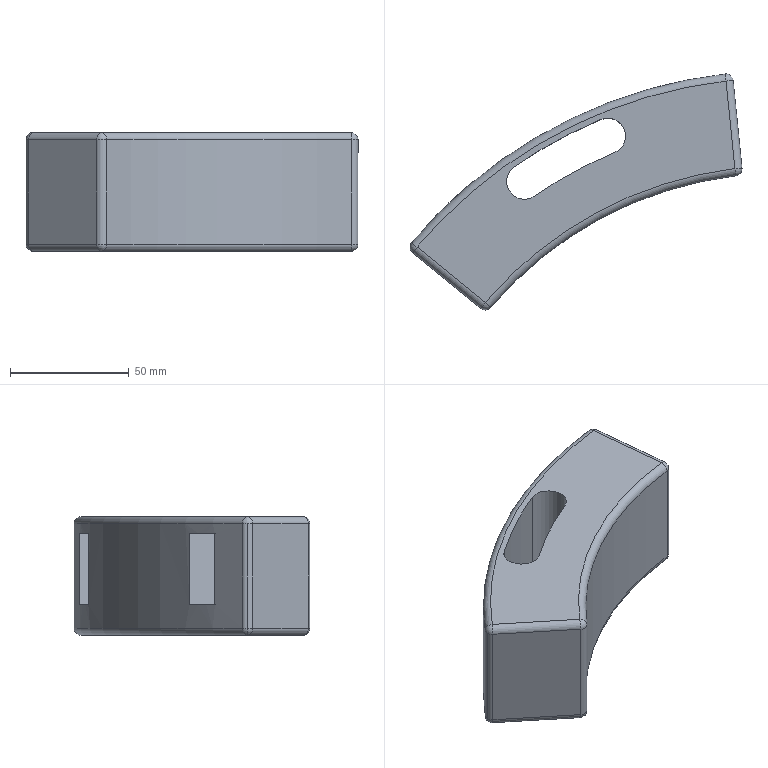Part | SolidWorks | features Cut 2, Extrusion 1, Fillet 1 | 1 solid | 44 faces | box 139.612 x 99.182 x 50 mm | volume 253889 mm3 | cylinder 16 | plane 14 | sphere 10 | torus 4 | commonest cylinder face diameters 6 x9 15 x3 319.919 x1 365 x1 395 x1 405.876 x1
STEP:
#1=CARTESIAN_POINT('',(-307.868,344.545,47.));
#2=VERTEX_POINT('',#1);
#3=CARTESIAN_POINT('',(-310.513,341.566,47.));
#4=VERTEX_POINT('',#3);
#5=CARTESIAN_POINT('',(-310.868,344.545,47.));
#6=DIRECTION('',(0.,0.,-1.));
#7=DIRECTION('',(1.,0.,0.));
#8=AXIS2_PLACEMENT_3D('',#5,#6,#7);
#9=CIRCLE('',#8,3.);
#10=EDGE_CURVE('',#2,#4,#9,.T.);
#11=ORIENTED_EDGE('',*,*,#10,.F.);
#12=CARTESIAN_POINT('',(-310.868,344.545,50.));
#13=VERTEX_POINT('',#12);
#14=CARTESIAN_POINT('',(-310.868,344.545,47.));
#15=DIRECTION('',(0.,-1.,0.));
#16=DIRECTION('',(1.,0.,0.));
#17=AXIS2_PLACEMENT_3D('',#14,#15,#16);
#18=CIRCLE('',#17,3.);
#19=EDGE_CURVE('',#2,#13,#18,.T.);
#20=ORIENTED_EDGE('',*,*,#19,.T.);
#21=CARTESIAN_POINT('',(-310.868,344.545,47.));
#22=DIRECTION('',(0.993,0.1183,0.));
#23=DIRECTION('',(-0.1183,0.993,0.));
#24=AXIS2_PLACEMENT_3D('',#21,#22,#23);
#25=CIRCLE('',#24,3.);
#26=EDGE_CURVE('',#13,#4,#25,.T.);
#27=ORIENTED_EDGE('',*,*,#26,.T.);
#28=EDGE_LOOP('',(#11,#20,#27));
#29=FACE_OUTER_BOUND('',#28,.T.);
#30=CARTESIAN_POINT('',(-310.868,344.545,47.));
#31=DIRECTION('',(0.,1.,0.));
#32=DIRECTION('',(1.,0.,0.));
#33=AXIS2_PLACEMENT_3D('',#30,#31,#32);
#34=SPHERICAL_SURFACE('',#33,3.);
#35=ADVANCED_FACE('',(#29),#34,.T.);
#36=CARTESIAN_POINT('',(-446.378,309.243,3.));
#37=VERTEX_POINT('',#36);
#38=CARTESIAN_POINT('',(-447.48,311.566,3.));
#39=VERTEX_POINT('',#38);
#40=CARTESIAN_POINT('',(-444.48,311.566,3.));
#41=DIRECTION('',(0.,0.,-1.));
#42=DIRECTION('',(-1.,0.,0.));
#43=AXIS2_PLACEMENT_3D('',#40,#41,#42);
#44=CIRCLE('',#43,3.);
#45=EDGE_CURVE('',#37,#39,#44,.T.);
#46=ORIENTED_EDGE('',*,*,#45,.T.);
#47=CARTESIAN_POINT('',(-444.48,311.566,0.));
#48=VERTEX_POINT('',#47);
#49=CARTESIAN_POINT('',(-444.48,311.566,3.));
#50=DIRECTION('',(0.,-1.,0.));
#51=DIRECTION('',(0.,0.,-1.));
#52=AXIS2_PLACEMENT_3D('',#49,#50,#51);
#53=CIRCLE('',#52,3.);
#54=EDGE_CURVE('',#39,#48,#53,.T.);
#55=ORIENTED_EDGE('',*,*,#54,.T.);
#56=CARTESIAN_POINT('',(-444.48,311.566,3.));
#57=DIRECTION('',(0.7743,-0.6328,0.));
#58=DIRECTION('',(-0.6328,-0.7743,0.));
#59=AXIS2_PLACEMENT_3D('',#56,#57,#58);
#60=CIRCLE('',#59,3.);
#61=EDGE_CURVE('',#37,#48,#60,.T.);
#62=ORIENTED_EDGE('',*,*,#61,.F.);
#63=EDGE_LOOP('',(#46,#55,#62));
#64=FACE_OUTER_BOUND('',#63,.T.);
#65=CARTESIAN_POINT('',(-444.48,311.566,3.));
#66=DIRECTION('',(0.,1.,0.));
#67=DIRECTION('',(-1.,0.,0.));
#68=AXIS2_PLACEMENT_3D('',#65,#66,#67);
#69=SPHERICAL_SURFACE('',#68,3.);
#70=ADVANCED_FACE('',(#64),#69,.T.);
#71=CARTESIAN_POINT('',(-446.378,309.243,47.));
#72=VERTEX_POINT('',#71);
#73=CARTESIAN_POINT('',(-447.48,311.566,47.));
#74=VERTEX_POINT('',#73);
#75=CARTESIAN_POINT('',(-444.48,311.566,47.));
#76=DIRECTION('',(0.,0.,-1.));
#77=DIRECTION('',(1.,0.,0.));
#78=AXIS2_PLACEMENT_3D('',#75,#76,#77);
#79=CIRCLE('',#78,3.);
#80=EDGE_CURVE('',#72,#74,#79,.T.);
#81=ORIENTED_EDGE('',*,*,#80,.T.);
#82=CARTESIAN_POINT('',(-447.48,311.566,50.));
#83=DIRECTION('',(0.,0.,-1.));
#84=VECTOR('',#83,1000.);
#85=LINE('',#82,#84);
#86=EDGE_CURVE('',#74,#39,#85,.T.);
#87=ORIENTED_EDGE('',*,*,#86,.T.);
#88=ORIENTED_EDGE('',*,*,#45,.F.);
#89=CARTESIAN_POINT('',(-446.378,309.243,50.));
#90=DIRECTION('',(0.,0.,-1.));
#91=VECTOR('',#90,1000.);
#92=LINE('',#89,#91);
#93=EDGE_CURVE('',#72,#37,#92,.T.);
#94=ORIENTED_EDGE('',*,*,#93,.F.);
#95=EDGE_LOOP('',(#81,#87,#88,#94));
#96=FACE_OUTER_BOUND('',#95,.T.);
#97=CARTESIAN_POINT('',(-444.48,311.566,50.));
#98=DIRECTION('',(0.,0.,-1.));
#99=DIRECTION('',(-1.,0.,0.));
#100=AXIS2_PLACEMENT_3D('',#97,#98,#99);
#101=CYLINDRICAL_SURFACE('',#100,3.);
#102=ADVANCED_FACE('',(#96),#101,.T.);
#103=CARTESIAN_POINT('',(-406.89,339.186,50.));
#104=VERTEX_POINT('',#103);
#105=CARTESIAN_POINT('',(-403.645,345.362,50.));
#106=VERTEX_POINT('',#105);
#107=CARTESIAN_POINT('',(-399.39,339.186,50.));
#108=DIRECTION('',(0.,0.,-1.));
#109=DIRECTION('',(-1.,0.,0.));
#110=AXIS2_PLACEMENT_3D('',#107,#108,#109);
#111=CIRCLE('',#110,7.5);
#112=EDGE_CURVE('',#104,#106,#111,.T.);
#113=ORIENTED_EDGE('',*,*,#112,.F.);
#114=CARTESIAN_POINT('',(-406.89,339.186,0.));
#115=VERTEX_POINT('',#114);
#116=CARTESIAN_POINT('',(-406.89,339.186,50.));
#117=DIRECTION('',(0.,0.,-1.));
#118=VECTOR('',#117,1000.);
#119=LINE('',#116,#118);
#120=EDGE_CURVE('',#104,#115,#119,.T.);
#121=ORIENTED_EDGE('',*,*,#120,.T.);
#122=CARTESIAN_POINT('',(-403.645,345.362,0.));
#123=VERTEX_POINT('',#122);
#124=CARTESIAN_POINT('',(-399.39,339.186,0.));
#125=DIRECTION('',(0.,0.,1.));
#126=DIRECTION('',(1.,0.,0.));
#127=AXIS2_PLACEMENT_3D('',#124,#125,#126);
#128=CIRCLE('',#127,7.5);
#129=EDGE_CURVE('',#123,#115,#128,.T.);
#130=ORIENTED_EDGE('',*,*,#129,.F.);
#131=CARTESIAN_POINT('',(-403.645,345.362,50.));
#132=DIRECTION('',(0.,0.,-1.));
#133=VECTOR('',#132,1000.);
#134=LINE('',#131,#133);
#135=EDGE_CURVE('',#106,#123,#134,.T.);
#136=ORIENTED_EDGE('',*,*,#135,.F.);
#137=EDGE_LOOP('',(#113,#121,#130,#136));
#138=FACE_OUTER_BOUND('',#137,.T.);
#139=CARTESIAN_POINT('',(-399.39,339.186,50.));
#140=DIRECTION('',(0.,0.,-1.));
#141=DIRECTION('',(-1.,0.,0.));
#142=AXIS2_PLACEMENT_3D('',#139,#140,#141);
#143=CYLINDRICAL_SURFACE('',#142,7.5);
#144=ADVANCED_FACE('',(#138),#143,.F.);
#145=CARTESIAN_POINT('',(-413.556,286.22,47.));
#146=VERTEX_POINT('',#145);
#147=CARTESIAN_POINT('',(-291.585,182.731,47.));
#148=DIRECTION('',(0.,0.,1.));
#149=DIRECTION('',(1.,0.,0.));
#150=AXIS2_PLACEMENT_3D('',#147,#148,#149);
#151=CIRCLE('',#150,159.959);
#152=EDGE_CURVE('',#4,#146,#151,.T.);
#153=ORIENTED_EDGE('',*,*,#152,.T.);
#154=CARTESIAN_POINT('',(-413.556,286.22,3.));
#155=VERTEX_POINT('',#154);
#156=CARTESIAN_POINT('',(-413.556,286.22,50.));
#157=DIRECTION('',(0.,0.,-1.));
#158=VECTOR('',#157,1000.);
#159=LINE('',#156,#158);
#160=EDGE_CURVE('',#146,#155,#159,.T.);
#161=ORIENTED_EDGE('',*,*,#160,.T.);
#162=CARTESIAN_POINT('',(-310.513,341.566,3.));
#163=VERTEX_POINT('',#162);
#164=CARTESIAN_POINT('',(-291.585,182.731,3.));
#165=DIRECTION('',(0.,0.,-1.));
#166=DIRECTION('',(1.,0.,0.));
#167=AXIS2_PLACEMENT_3D('',#164,#165,#166);
#168=CIRCLE('',#167,159.959);
#169=EDGE_CURVE('',#155,#163,#168,.T.);
#170=ORIENTED_EDGE('',*,*,#169,.T.);
#171=CARTESIAN_POINT('',(-310.513,341.566,50.));
#172=DIRECTION('',(0.,0.,1.));
#173=VECTOR('',#172,1000.);
#174=LINE('',#171,#173);
#175=EDGE_CURVE('',#163,#4,#174,.T.);
#176=ORIENTED_EDGE('',*,*,#175,.T.);
#177=EDGE_LOOP('',(#153,#161,#170,#176));
#178=FACE_OUTER_BOUND('',#177,.T.);
#179=CARTESIAN_POINT('',(-291.585,182.731,50.));
#180=DIRECTION('',(0.,0.,-1.));
#181=DIRECTION('',(-1.,0.,0.));
#182=AXIS2_PLACEMENT_3D('',#179,#180,#181);
#183=CYLINDRICAL_SURFACE('',#182,159.959);
#184=ADVANCED_FACE('',(#178),#183,.F.);
#185=CARTESIAN_POINT('',(-307.883,344.845,3.));
#186=VERTEX_POINT('',#185);
#187=CARTESIAN_POINT('',(-311.583,381.644,3.));
#188=VERTEX_POINT('',#187);
#189=CARTESIAN_POINT('',(-307.586,341.888,3.));
#190=DIRECTION('',(-0.1,0.995,0.));
#191=VECTOR('',#190,1000.);
#192=LINE('',#189,#191);
#193=EDGE_CURVE('',#186,#188,#192,.T.);
#194=ORIENTED_EDGE('',*,*,#193,.T.);
#195=CARTESIAN_POINT('',(-311.583,381.644,47.));
#196=VERTEX_POINT('',#195);
#197=CARTESIAN_POINT('',(-311.583,381.644,50.));
#198=DIRECTION('',(0.,0.,1.));
#199=VECTOR('',#198,1000.);
#200=LINE('',#197,#199);
#201=EDGE_CURVE('',#188,#196,#200,.T.);
#202=ORIENTED_EDGE('',*,*,#201,.T.);
#203=CARTESIAN_POINT('',(-307.883,344.845,47.));
#204=VERTEX_POINT('',#203);
#205=CARTESIAN_POINT('',(-307.586,341.888,47.));
#206=DIRECTION('',(0.1,-0.995,0.));
#207=VECTOR('',#206,1000.);
#208=LINE('',#205,#207);
#209=EDGE_CURVE('',#196,#204,#208,.T.);
#210=ORIENTED_EDGE('',*,*,#209,.T.);
#211=CARTESIAN_POINT('',(-307.883,344.845,50.));
#212=DIRECTION('',(0.,0.,-1.));
#213=VECTOR('',#212,1000.);
#214=LINE('',#211,#213);
#215=EDGE_CURVE('',#204,#186,#214,.T.);
#216=ORIENTED_EDGE('',*,*,#215,.T.);
#217=EDGE_LOOP('',(#194,#202,#210,#216));
#218=FACE_OUTER_BOUND('',#217,.T.);
#219=CARTESIAN_POINT('',(-307.586,341.888,50.));
#220=DIRECTION('',(-0.995,-0.1,0.));
#221=DIRECTION('',(0.1,-0.995,0.));
#222=AXIS2_PLACEMENT_3D('',#219,#220,#221);
#223=PLANE('',#222);
#224=ADVANCED_FACE('',(#218),#223,.F.);
#225=CARTESIAN_POINT('',(-314.913,384.324,3.));
#226=VERTEX_POINT('',#225);
#227=CARTESIAN_POINT('',(-446.774,313.499,3.));
#228=VERTEX_POINT('',#227);
#229=CARTESIAN_POINT('',(-291.585,182.731,3.));
#230=DIRECTION('',(0.,0.,1.));
#231=DIRECTION('',(1.,0.,0.));
#232=AXIS2_PLACEMENT_3D('',#229,#230,#231);
#233=CIRCLE('',#232,202.938);
#234=EDGE_CURVE('',#226,#228,#233,.T.);
#235=ORIENTED_EDGE('',*,*,#234,.T.);
#236=CARTESIAN_POINT('',(-446.774,313.499,47.));
#237=VERTEX_POINT('',#236);
#238=CARTESIAN_POINT('',(-446.774,313.499,50.));
#239=DIRECTION('',(0.,0.,1.));
#240=VECTOR('',#239,1000.);
#241=LINE('',#238,#240);
#242=EDGE_CURVE('',#228,#237,#241,.T.);
#243=ORIENTED_EDGE('',*,*,#242,.T.);
#244=CARTESIAN_POINT('',(-314.913,384.324,47.));
#245=VERTEX_POINT('',#244);
#246=CARTESIAN_POINT('',(-291.585,182.731,47.));
#247=DIRECTION('',(0.,0.,-1.));
#248=DIRECTION('',(1.,0.,0.));
#249=AXIS2_PLACEMENT_3D('',#246,#247,#248);
#250=CIRCLE('',#249,202.938);
#251=EDGE_CURVE('',#237,#245,#250,.T.);
#252=ORIENTED_EDGE('',*,*,#251,.T.);
#253=CARTESIAN_POINT('',(-314.913,384.324,50.));
#254=DIRECTION('',(0.,0.,-1.));
#255=VECTOR('',#254,1000.);
#256=LINE('',#253,#255);
#257=EDGE_CURVE('',#245,#226,#256,.T.);
#258=ORIENTED_EDGE('',*,*,#257,.T.);
#259=EDGE_LOOP('',(#235,#243,#252,#258));
#260=FACE_OUTER_BOUND('',#259,.T.);
#261=CARTESIAN_POINT('',(-424.864,335.768,43.));
#262=VERTEX_POINT('',#261);
#263=CARTESIAN_POINT('',(-436.176,325.129,43.));
#264=VERTEX_POINT('',#263);
#265=CARTESIAN_POINT('',(-291.585,182.731,43.));
#266=DIRECTION('',(0.,0.,1.));
#267=DIRECTION('',(1.,0.,0.));
#268=AXIS2_PLACEMENT_3D('',#265,#266,#267);
#269=CIRCLE('',#268,202.938);
#270=EDGE_CURVE('',#262,#264,#269,.T.);
#271=ORIENTED_EDGE('',*,*,#270,.T.);
#272=CARTESIAN_POINT('',(-436.176,325.129,13.));
#273=VERTEX_POINT('',#272);
#274=CARTESIAN_POINT('',(-436.176,325.129,50.));
#275=DIRECTION('',(0.,0.,-1.));
#276=VECTOR('',#275,1000.);
#277=LINE('',#274,#276);
#278=EDGE_CURVE('',#264,#273,#277,.T.);
#279=ORIENTED_EDGE('',*,*,#278,.T.);
#280=CARTESIAN_POINT('',(-424.864,335.768,13.));
#281=VERTEX_POINT('',#280);
#282=CARTESIAN_POINT('',(-291.585,182.731,13.));
#283=DIRECTION('',(0.,0.,-1.));
#284=DIRECTION('',(-1.,0.,0.));
#285=AXIS2_PLACEMENT_3D('',#282,#283,#284);
#286=CIRCLE('',#285,202.938);
#287=EDGE_CURVE('',#273,#281,#286,.T.);
#288=ORIENTED_EDGE('',*,*,#287,.T.);
#289=CARTESIAN_POINT('',(-424.864,335.768,50.));
#290=DIRECTION('',(0.,0.,1.));
#291=VECTOR('',#290,1000.);
#292=LINE('',#289,#291);
#293=EDGE_CURVE('',#281,#262,#292,.T.);
#294=ORIENTED_EDGE('',*,*,#293,.T.);
#295=EDGE_LOOP('',(#271,#279,#288,#294));
#296=FACE_BOUND('',#295,.T.);
#297=CARTESIAN_POINT('',(-330.461,381.91,43.));
#298=VERTEX_POINT('',#297);
#299=CARTESIAN_POINT('',(-345.577,378.355,43.));
#300=VERTEX_POINT('',#299);
#301=CARTESIAN_POINT('',(-291.585,182.731,43.));
#302=DIRECTION('',(0.,0.,1.));
#303=DIRECTION('',(1.,0.,0.));
#304=AXIS2_PLACEMENT_3D('',#301,#302,#303);
#305=CIRCLE('',#304,202.938);
#306=EDGE_CURVE('',#298,#300,#305,.T.);
#307=ORIENTED_EDGE('',*,*,#306,.T.);
#308=CARTESIAN_POINT('',(-345.577,378.355,13.));
#309=VERTEX_POINT('',#308);
#310=CARTESIAN_POINT('',(-345.577,378.355,50.));
#311=DIRECTION('',(0.,0.,-1.));
#312=VECTOR('',#311,1000.);
#313=LINE('',#310,#312);
#314=EDGE_CURVE('',#300,#309,#313,.T.);
#315=ORIENTED_EDGE('',*,*,#314,.T.);
#316=CARTESIAN_POINT('',(-330.461,381.91,13.));
#317=VERTEX_POINT('',#316);
#318=CARTESIAN_POINT('',(-291.585,182.731,13.));
#319=DIRECTION('',(0.,0.,-1.));
#320=DIRECTION('',(-1.,0.,0.));
#321=AXIS2_PLACEMENT_3D('',#318,#319,#320);
#322=CIRCLE('',#321,202.938);
#323=EDGE_CURVE('',#309,#317,#322,.T.);
#324=ORIENTED_EDGE('',*,*,#323,.T.);
#325=CARTESIAN_POINT('',(-330.461,381.91,50.));
#326=DIRECTION('',(0.,0.,1.));
#327=VECTOR('',#326,1000.);
#328=LINE('',#325,#327);
#329=EDGE_CURVE('',#317,#298,#328,.T.);
#330=ORIENTED_EDGE('',*,*,#329,.T.);
#331=EDGE_LOOP('',(#307,#315,#324,#330));
#332=FACE_BOUND('',#331,.T.);
#333=CARTESIAN_POINT('',(-291.585,182.731,50.));
#334=DIRECTION('',(0.,0.,-1.));
#335=DIRECTION('',(-1.,0.,0.));
#336=AXIS2_PLACEMENT_3D('',#333,#334,#335);
#337=CYLINDRICAL_SURFACE('',#336,202.938);
#338=ADVANCED_FACE('',(#260,#296,#332),#337,.T.);
#339=ORIENTED_EDGE('',*,*,#93,.T.);
#340=CARTESIAN_POINT('',(-417.742,285.839,3.));
#341=VERTEX_POINT('',#340);
#342=CARTESIAN_POINT('',(-415.441,283.958,3.));
#343=DIRECTION('',(0.7743,-0.6328,0.));
#344=VECTOR('',#343,1000.);
#345=LINE('',#342,#344);
#346=EDGE_CURVE('',#37,#341,#345,.T.);
#347=ORIENTED_EDGE('',*,*,#346,.T.);
#348=CARTESIAN_POINT('',(-417.742,285.839,47.));
#349=VERTEX_POINT('',#348);
#350=CARTESIAN_POINT('',(-417.742,285.839,50.));
#351=DIRECTION('',(0.,0.,1.));
#352=VECTOR('',#351,1000.);
#353=LINE('',#350,#352);
#354=EDGE_CURVE('',#341,#349,#353,.T.);
#355=ORIENTED_EDGE('',*,*,#354,.T.);
#356=CARTESIAN_POINT('',(-448.719,311.156,47.));
#357=DIRECTION('',(-0.7743,0.6328,0.));
#358=VECTOR('',#357,1000.);
#359=LINE('',#356,#358);
#360=EDGE_CURVE('',#349,#72,#359,.T.);
#361=ORIENTED_EDGE('',*,*,#360,.T.);
#362=EDGE_LOOP('',(#339,#347,#355,#361));
#363=FACE_OUTER_BOUND('',#362,.T.);
#364=CARTESIAN_POINT('',(-415.441,283.958,50.));
#365=DIRECTION('',(0.6328,0.7743,0.));
#366=DIRECTION('',(-0.7743,0.6328,0.));
#367=AXIS2_PLACEMENT_3D('',#364,#365,#366);
#368=PLANE('',#367);
#369=ADVANCED_FACE('',(#363),#368,.F.);
#370=CARTESIAN_POINT('',(-444.48,311.566,50.));
#371=VERTEX_POINT('',#370);
#372=CARTESIAN_POINT('',(-415.844,288.161,50.));
#373=VERTEX_POINT('',#372);
#374=CARTESIAN_POINT('',(-413.542,286.28,50.));
#375=DIRECTION('',(0.7743,-0.6328,0.));
#376=VECTOR('',#375,1000.);
#377=LINE('',#374,#376);
#378=EDGE_CURVE('',#371,#373,#377,.T.);
#379=ORIENTED_EDGE('',*,*,#378,.T.);
#380=CARTESIAN_POINT('',(-291.585,182.731,50.));
#381=DIRECTION('',(0.,0.,-1.));
#382=DIRECTION('',(1.,0.,0.));
#383=AXIS2_PLACEMENT_3D('',#380,#381,#382);
#384=CIRCLE('',#383,162.959);
#385=EDGE_CURVE('',#373,#13,#384,.T.);
#386=ORIENTED_EDGE('',*,*,#385,.T.);
#387=CARTESIAN_POINT('',(-314.568,381.343,50.));
#388=VERTEX_POINT('',#387);
#389=CARTESIAN_POINT('',(-314.87,384.351,50.));
#390=DIRECTION('',(-0.1,0.995,0.));
#391=VECTOR('',#390,1000.);
#392=LINE('',#389,#391);
#393=EDGE_CURVE('',#13,#388,#392,.T.);
#394=ORIENTED_EDGE('',*,*,#393,.T.);
#395=CARTESIAN_POINT('',(-291.585,182.731,50.));
#396=DIRECTION('',(0.,0.,1.));
#397=DIRECTION('',(1.,0.,0.));
#398=AXIS2_PLACEMENT_3D('',#395,#396,#397);
#399=CIRCLE('',#398,199.938);
#400=EDGE_CURVE('',#388,#371,#399,.T.);
#401=ORIENTED_EDGE('',*,*,#400,.T.);
#402=EDGE_LOOP('',(#379,#386,#394,#401));
#403=FACE_OUTER_BOUND('',#402,.T.);
#404=CARTESIAN_POINT('',(-395.134,333.01,50.));
#405=VERTEX_POINT('',#404);
#406=CARTESIAN_POINT('',(-399.39,339.186,50.));
#407=DIRECTION('',(0.,0.,-1.));
#408=DIRECTION('',(-1.,0.,0.));
#409=AXIS2_PLACEMENT_3D('',#406,#407,#408);
#410=CIRCLE('',#409,7.5);
#411=EDGE_CURVE('',#405,#104,#410,.T.);
#412=ORIENTED_EDGE('',*,*,#411,.T.);
#413=ORIENTED_EDGE('',*,*,#112,.T.);
#414=CARTESIAN_POINT('',(-367.185,365.189,50.));
#415=VERTEX_POINT('',#414);
#416=CARTESIAN_POINT('',(-291.585,182.731,50.));
#417=DIRECTION('',(0.,0.,-1.));
#418=DIRECTION('',(-1.,0.,0.));
#419=AXIS2_PLACEMENT_3D('',#416,#417,#418);
#420=CIRCLE('',#419,197.5);
#421=EDGE_CURVE('',#106,#415,#420,.T.);
#422=ORIENTED_EDGE('',*,*,#421,.T.);
#423=CARTESIAN_POINT('',(-361.443,351.331,50.));
#424=VERTEX_POINT('',#423);
#425=CARTESIAN_POINT('',(-364.314,358.26,50.));
#426=DIRECTION('',(0.,0.,-1.));
#427=DIRECTION('',(-1.,0.,0.));
#428=AXIS2_PLACEMENT_3D('',#425,#426,#427);
#429=CIRCLE('',#428,7.5);
#430=EDGE_CURVE('',#415,#424,#429,.T.);
#431=ORIENTED_EDGE('',*,*,#430,.T.);
#432=CARTESIAN_POINT('',(-291.585,182.731,50.));
#433=DIRECTION('',(0.,0.,1.));
#434=DIRECTION('',(-1.,0.,0.));
#435=AXIS2_PLACEMENT_3D('',#432,#433,#434);
#436=CIRCLE('',#435,182.5);
#437=EDGE_CURVE('',#424,#405,#436,.T.);
#438=ORIENTED_EDGE('',*,*,#437,.T.);
#439=EDGE_LOOP('',(#412,#413,#422,#431,#438));
#440=FACE_BOUND('',#439,.T.);
#441=CARTESIAN_POINT('',(-291.585,182.731,50.));
#442=DIRECTION('',(0.,0.,1.));
#443=DIRECTION('',(1.,0.,0.));
#444=AXIS2_PLACEMENT_3D('',#441,#442,#443);
#445=PLANE('',#444);
#446=ADVANCED_FACE('',(#403,#440),#445,.T.);
#447=CARTESIAN_POINT('',(-314.568,381.343,0.));
#448=VERTEX_POINT('',#447);
#449=CARTESIAN_POINT('',(-310.868,344.545,0.));
#450=VERTEX_POINT('',#449);
#451=CARTESIAN_POINT('',(-294.57,182.431,0.));
#452=DIRECTION('',(0.1,-0.995,0.));
#453=VECTOR('',#452,1000.);
#454=LINE('',#451,#453);
#455=EDGE_CURVE('',#448,#450,#454,.T.);
#456=ORIENTED_EDGE('',*,*,#455,.T.);
#457=CARTESIAN_POINT('',(-415.844,288.161,0.));
#458=VERTEX_POINT('',#457);
#459=CARTESIAN_POINT('',(-291.585,182.731,0.));
#460=DIRECTION('',(0.,0.,1.));
#461=DIRECTION('',(1.,0.,0.));
#462=AXIS2_PLACEMENT_3D('',#459,#460,#461);
#463=CIRCLE('',#462,162.959);
#464=EDGE_CURVE('',#450,#458,#463,.T.);
#465=ORIENTED_EDGE('',*,*,#464,.T.);
#466=CARTESIAN_POINT('',(-289.687,185.054,0.));
#467=DIRECTION('',(-0.7743,0.6328,0.));
#468=VECTOR('',#467,1000.);
#469=LINE('',#466,#468);
#470=EDGE_CURVE('',#458,#48,#469,.T.);
#471=ORIENTED_EDGE('',*,*,#470,.T.);
#472=CARTESIAN_POINT('',(-291.585,182.731,0.));
#473=DIRECTION('',(0.,0.,-1.));
#474=DIRECTION('',(1.,0.,0.));
#475=AXIS2_PLACEMENT_3D('',#472,#473,#474);
#476=CIRCLE('',#475,199.938);
#477=EDGE_CURVE('',#48,#448,#476,.T.);
#478=ORIENTED_EDGE('',*,*,#477,.T.);
#479=EDGE_LOOP('',(#456,#465,#471,#478));
#480=FACE_OUTER_BOUND('',#479,.T.);
#481=CARTESIAN_POINT('',(-367.185,365.189,0.));
#482=VERTEX_POINT('',#481);
#483=CARTESIAN_POINT('',(-291.585,182.731,0.));
#484=DIRECTION('',(0.,0.,1.));
#485=DIRECTION('',(1.,0.,0.));
#486=AXIS2_PLACEMENT_3D('',#483,#484,#485);
#487=CIRCLE('',#486,197.5);
#488=EDGE_CURVE('',#482,#123,#487,.T.);
#489=ORIENTED_EDGE('',*,*,#488,.T.);
#490=ORIENTED_EDGE('',*,*,#129,.T.);
#491=CARTESIAN_POINT('',(-395.134,333.01,0.));
#492=VERTEX_POINT('',#491);
#493=CARTESIAN_POINT('',(-399.39,339.186,0.));
#494=DIRECTION('',(0.,0.,1.));
#495=DIRECTION('',(1.,0.,0.));
#496=AXIS2_PLACEMENT_3D('',#493,#494,#495);
#497=CIRCLE('',#496,7.5);
#498=EDGE_CURVE('',#115,#492,#497,.T.);
#499=ORIENTED_EDGE('',*,*,#498,.T.);
#500=CARTESIAN_POINT('',(-361.443,351.331,0.));
#501=VERTEX_POINT('',#500);
#502=CARTESIAN_POINT('',(-291.585,182.731,0.));
#503=DIRECTION('',(0.,0.,-1.));
#504=DIRECTION('',(1.,0.,0.));
#505=AXIS2_PLACEMENT_3D('',#502,#503,#504);
#506=CIRCLE('',#505,182.5);
#507=EDGE_CURVE('',#492,#501,#506,.T.);
#508=ORIENTED_EDGE('',*,*,#507,.T.);
#509=CARTESIAN_POINT('',(-364.314,358.26,0.));
#510=DIRECTION('',(0.,0.,1.));
#511=DIRECTION('',(1.,0.,0.));
#512=AXIS2_PLACEMENT_3D('',#509,#510,#511);
#513=CIRCLE('',#512,7.5);
#514=EDGE_CURVE('',#501,#482,#513,.T.);
#515=ORIENTED_EDGE('',*,*,#514,.T.);
#516=EDGE_LOOP('',(#489,#490,#499,#508,#515));
#517=FACE_BOUND('',#516,.T.);
#518=CARTESIAN_POINT('',(-291.585,182.731,0.));
#519=DIRECTION('',(0.,0.,1.));
#520=DIRECTION('',(1.,0.,0.));
#521=AXIS2_PLACEMENT_3D('',#518,#519,#520);
#522=PLANE('',#521);
#523=ADVANCED_FACE('',(#480,#517),#522,.F.);
#524=CARTESIAN_POINT('',(-338.504,365.186,43.));
#525=VERTEX_POINT('',#524);
#526=CARTESIAN_POINT('',(-338.504,365.186,43.));
#527=DIRECTION('',(-0.4732,0.881,0.));
#528=VECTOR('',#527,1000.);
#529=LINE('',#526,#528);
#530=EDGE_CURVE('',#525,#300,#529,.T.);
#531=ORIENTED_EDGE('',*,*,#530,.F.);
#532=CARTESIAN_POINT('',(-338.504,365.186,13.));
#533=VERTEX_POINT('',#532);
#534=CARTESIAN_POINT('',(-338.504,365.186,43.));
#535=DIRECTION('',(0.,0.,1.));
#536=VECTOR('',#535,1000.);
#537=LINE('',#534,#536);
#538=EDGE_CURVE('',#533,#525,#537,.T.);
#539=ORIENTED_EDGE('',*,*,#538,.F.);
#540=CARTESIAN_POINT('',(-338.504,365.186,13.));
#541=DIRECTION('',(-0.4732,0.881,0.));
#542=VECTOR('',#541,1000.);
#543=LINE('',#540,#542);
#544=EDGE_CURVE('',#533,#309,#543,.T.);
#545=ORIENTED_EDGE('',*,*,#544,.T.);
#546=ORIENTED_EDGE('',*,*,#314,.F.);
#547=EDGE_LOOP('',(#531,#539,#545,#546));
#548=FACE_OUTER_BOUND('',#547,.T.);
#549=CARTESIAN_POINT('',(-338.504,365.186,43.));
#550=DIRECTION('',(-0.881,-0.4732,0.));
#551=DIRECTION('',(0.4732,-0.881,0.));
#552=AXIS2_PLACEMENT_3D('',#549,#550,#551);
#553=PLANE('',#552);
#554=ADVANCED_FACE('',(#548),#553,.F.);
#555=ORIENTED_EDGE('',*,*,#544,.F.);
#556=CARTESIAN_POINT('',(-325.29,372.284,13.));
#557=VERTEX_POINT('',#556);
#558=CARTESIAN_POINT('',(-325.29,372.284,13.));
#559=DIRECTION('',(-0.881,-0.4732,0.));
#560=VECTOR('',#559,1000.);
#561=LINE('',#558,#560);
#562=EDGE_CURVE('',#557,#533,#561,.T.);
#563=ORIENTED_EDGE('',*,*,#562,.F.);
#564=CARTESIAN_POINT('',(-325.29,372.284,13.));
#565=DIRECTION('',(-0.4732,0.881,0.));
#566=VECTOR('',#565,1000.);
#567=LINE('',#564,#566);
#568=EDGE_CURVE('',#557,#317,#567,.T.);
#569=ORIENTED_EDGE('',*,*,#568,.T.);
#570=ORIENTED_EDGE('',*,*,#323,.F.);
#571=EDGE_LOOP('',(#555,#563,#569,#570));
#572=FACE_OUTER_BOUND('',#571,.T.);
#573=CARTESIAN_POINT('',(-325.29,372.284,13.));
#574=DIRECTION('',(0.,0.,-1.));
#575=DIRECTION('',(-1.,0.,0.));
#576=AXIS2_PLACEMENT_3D('',#573,#574,#575);
#577=PLANE('',#576);
#578=ADVANCED_FACE('',(#572),#577,.F.);
#579=ORIENTED_EDGE('',*,*,#568,.F.);
#580=CARTESIAN_POINT('',(-325.29,372.284,43.));
#581=VERTEX_POINT('',#580);
#582=CARTESIAN_POINT('',(-325.29,372.284,43.));
#583=DIRECTION('',(0.,0.,-1.));
#584=VECTOR('',#583,1000.);
#585=LINE('',#582,#584);
#586=EDGE_CURVE('',#581,#557,#585,.T.);
#587=ORIENTED_EDGE('',*,*,#586,.F.);
#588=CARTESIAN_POINT('',(-325.29,372.284,43.));
#589=DIRECTION('',(-0.4732,0.881,0.));
#590=VECTOR('',#589,1000.);
#591=LINE('',#588,#590);
#592=EDGE_CURVE('',#581,#298,#591,.T.);
#593=ORIENTED_EDGE('',*,*,#592,.T.);
#594=ORIENTED_EDGE('',*,*,#329,.F.);
#595=EDGE_LOOP('',(#579,#587,#593,#594));
#596=FACE_OUTER_BOUND('',#595,.T.);
#597=CARTESIAN_POINT('',(-325.29,372.284,43.));
#598=DIRECTION('',(0.881,0.4732,0.));
#599=DIRECTION('',(-0.4732,0.881,0.));
#600=AXIS2_PLACEMENT_3D('',#597,#598,#599);
#601=PLANE('',#600);
#602=ADVANCED_FACE('',(#596),#601,.F.);
#603=ORIENTED_EDGE('',*,*,#592,.F.);
#604=CARTESIAN_POINT('',(-325.29,372.284,43.));
#605=DIRECTION('',(0.881,0.4732,0.));
#606=VECTOR('',#605,1000.);
#607=LINE('',#604,#606);
#608=EDGE_CURVE('',#525,#581,#607,.T.);
#609=ORIENTED_EDGE('',*,*,#608,.F.);
#610=ORIENTED_EDGE('',*,*,#530,.T.);
#611=ORIENTED_EDGE('',*,*,#306,.F.);
#612=EDGE_LOOP('',(#603,#609,#610,#611));
#613=FACE_OUTER_BOUND('',#612,.T.);
#614=CARTESIAN_POINT('',(-325.29,372.284,43.));
#615=DIRECTION('',(0.,0.,1.));
#616=DIRECTION('',(1.,0.,0.));
#617=AXIS2_PLACEMENT_3D('',#614,#615,#616);
#618=PLANE('',#617);
#619=ADVANCED_FACE('',(#613),#618,.F.);
#620=ORIENTED_EDGE('',*,*,#538,.T.);
#621=ORIENTED_EDGE('',*,*,#608,.T.);
#622=ORIENTED_EDGE('',*,*,#586,.T.);
#623=ORIENTED_EDGE('',*,*,#562,.T.);
#624=EDGE_LOOP('',(#620,#621,#622,#623));
#625=FACE_OUTER_BOUND('',#624,.T.);
#626=CARTESIAN_POINT('',(-228.02,424.528,0.));
#627=DIRECTION('',(-0.4732,0.881,0.));
#628=DIRECTION('',(-0.881,-0.4732,0.));
#629=AXIS2_PLACEMENT_3D('',#626,#627,#628);
#630=PLANE('',#629);
#631=ADVANCED_FACE('',(#625),#630,.T.);
#632=CARTESIAN_POINT('',(-431.006,315.502,43.));
#633=VERTEX_POINT('',#632);
#634=CARTESIAN_POINT('',(-431.006,315.502,43.));
#635=DIRECTION('',(-0.4732,0.881,0.));
#636=VECTOR('',#635,1000.);
#637=LINE('',#634,#636);
#638=EDGE_CURVE('',#633,#264,#637,.T.);
#639=ORIENTED_EDGE('',*,*,#638,.F.);
#640=CARTESIAN_POINT('',(-431.006,315.502,13.));
#641=VERTEX_POINT('',#640);
#642=CARTESIAN_POINT('',(-431.006,315.502,43.));
#643=DIRECTION('',(0.,0.,1.));
#644=VECTOR('',#643,1000.);
#645=LINE('',#642,#644);
#646=EDGE_CURVE('',#641,#633,#645,.T.);
#647=ORIENTED_EDGE('',*,*,#646,.F.);
#648=CARTESIAN_POINT('',(-431.006,315.502,13.));
#649=DIRECTION('',(-0.4732,0.881,0.));
#650=VECTOR('',#649,1000.);
#651=LINE('',#648,#650);
#652=EDGE_CURVE('',#641,#273,#651,.T.);
#653=ORIENTED_EDGE('',*,*,#652,.T.);
#654=ORIENTED_EDGE('',*,*,#278,.F.);
#655=EDGE_LOOP('',(#639,#647,#653,#654));
#656=FACE_OUTER_BOUND('',#655,.T.);
#657=CARTESIAN_POINT('',(-431.006,315.502,43.));
#658=DIRECTION('',(-0.881,-0.4732,0.));
#659=DIRECTION('',(0.4732,-0.881,0.));
#660=AXIS2_PLACEMENT_3D('',#657,#658,#659);
#661=PLANE('',#660);
#662=ADVANCED_FACE('',(#656),#661,.F.);
#663=ORIENTED_EDGE('',*,*,#652,.F.);
#664=CARTESIAN_POINT('',(-417.791,322.6,13.));
#665=VERTEX_POINT('',#664);
#666=CARTESIAN_POINT('',(-417.791,322.6,13.));
#667=DIRECTION('',(-0.881,-0.4732,0.));
#668=VECTOR('',#667,1000.);
#669=LINE('',#666,#668);
#670=EDGE_CURVE('',#665,#641,#669,.T.);
#671=ORIENTED_EDGE('',*,*,#670,.F.);
#672=CARTESIAN_POINT('',(-417.791,322.6,13.));
#673=DIRECTION('',(-0.4732,0.881,0.));
#674=VECTOR('',#673,1000.);
#675=LINE('',#672,#674);
#676=EDGE_CURVE('',#665,#281,#675,.T.);
#677=ORIENTED_EDGE('',*,*,#676,.T.);
#678=ORIENTED_EDGE('',*,*,#287,.F.);
#679=EDGE_LOOP('',(#663,#671,#677,#678));
#680=FACE_OUTER_BOUND('',#679,.T.);
#681=CARTESIAN_POINT('',(-417.791,322.6,13.));
#682=DIRECTION('',(0.,0.,-1.));
#683=DIRECTION('',(-1.,0.,0.));
#684=AXIS2_PLACEMENT_3D('',#681,#682,#683);
#685=PLANE('',#684);
#686=ADVANCED_FACE('',(#680),#685,.F.);
#687=ORIENTED_EDGE('',*,*,#676,.F.);
#688=CARTESIAN_POINT('',(-417.791,322.6,43.));
#689=VERTEX_POINT('',#688);
#690=CARTESIAN_POINT('',(-417.791,322.6,43.));
#691=DIRECTION('',(0.,0.,-1.));
#692=VECTOR('',#691,1000.);
#693=LINE('',#690,#692);
#694=EDGE_CURVE('',#689,#665,#693,.T.);
#695=ORIENTED_EDGE('',*,*,#694,.F.);
#696=CARTESIAN_POINT('',(-417.791,322.6,43.));
#697=DIRECTION('',(-0.4732,0.881,0.));
#698=VECTOR('',#697,1000.);
#699=LINE('',#696,#698);
#700=EDGE_CURVE('',#689,#262,#699,.T.);
#701=ORIENTED_EDGE('',*,*,#700,.T.);
#702=ORIENTED_EDGE('',*,*,#293,.F.);
#703=EDGE_LOOP('',(#687,#695,#701,#702));
#704=FACE_OUTER_BOUND('',#703,.T.);
#705=CARTESIAN_POINT('',(-417.791,322.6,43.));
#706=DIRECTION('',(0.881,0.4732,0.));
#707=DIRECTION('',(-0.4732,0.881,0.));
#708=AXIS2_PLACEMENT_3D('',#705,#706,#707);
#709=PLANE('',#708);
#710=ADVANCED_FACE('',(#704),#709,.F.);
#711=ORIENTED_EDGE('',*,*,#700,.F.);
#712=CARTESIAN_POINT('',(-417.791,322.6,43.));
#713=DIRECTION('',(0.881,0.4732,0.));
#714=VECTOR('',#713,1000.);
#715=LINE('',#712,#714);
#716=EDGE_CURVE('',#633,#689,#715,.T.);
#717=ORIENTED_EDGE('',*,*,#716,.F.);
#718=ORIENTED_EDGE('',*,*,#638,.T.);
#719=ORIENTED_EDGE('',*,*,#270,.F.);
#720=EDGE_LOOP('',(#711,#717,#718,#719));
#721=FACE_OUTER_BOUND('',#720,.T.);
#722=CARTESIAN_POINT('',(-417.791,322.6,43.));
#723=DIRECTION('',(0.,0.,1.));
#724=DIRECTION('',(1.,0.,0.));
#725=AXIS2_PLACEMENT_3D('',#722,#723,#724);
#726=PLANE('',#725);
#727=ADVANCED_FACE('',(#721),#726,.F.);
#728=ORIENTED_EDGE('',*,*,#646,.T.);
#729=ORIENTED_EDGE('',*,*,#716,.T.);
#730=ORIENTED_EDGE('',*,*,#694,.T.);
#731=ORIENTED_EDGE('',*,*,#670,.T.);
#732=EDGE_LOOP('',(#728,#729,#730,#731));
#733=FACE_OUTER_BOUND('',#732,.T.);
#734=CARTESIAN_POINT('',(-228.02,424.528,0.));
#735=DIRECTION('',(-0.4732,0.881,0.));
#736=DIRECTION('',(-0.881,-0.4732,0.));
#737=AXIS2_PLACEMENT_3D('',#734,#735,#736);
#738=PLANE('',#737);
#739=ADVANCED_FACE('',(#733),#738,.T.);
#740=ORIENTED_EDGE('',*,*,#120,.F.);
#741=ORIENTED_EDGE('',*,*,#411,.F.);
#742=CARTESIAN_POINT('',(-395.134,333.01,50.));
#743=DIRECTION('',(0.,0.,-1.));
#744=VECTOR('',#743,1000.);
#745=LINE('',#742,#744);
#746=EDGE_CURVE('',#405,#492,#745,.T.);
#747=ORIENTED_EDGE('',*,*,#746,.T.);
#748=ORIENTED_EDGE('',*,*,#498,.F.);
#749=EDGE_LOOP('',(#740,#741,#747,#748));
#750=FACE_OUTER_BOUND('',#749,.T.);
#751=CARTESIAN_POINT('',(-399.39,339.186,50.));
#752=DIRECTION('',(0.,0.,-1.));
#753=DIRECTION('',(-1.,0.,0.));
#754=AXIS2_PLACEMENT_3D('',#751,#752,#753);
#755=CYLINDRICAL_SURFACE('',#754,7.5);
#756=ADVANCED_FACE('',(#750),#755,.F.);
#757=ORIENTED_EDGE('',*,*,#746,.F.);
#758=ORIENTED_EDGE('',*,*,#437,.F.);
#759=CARTESIAN_POINT('',(-361.443,351.331,50.));
#760=DIRECTION('',(0.,0.,-1.));
#761=VECTOR('',#760,1000.);
#762=LINE('',#759,#761);
#763=EDGE_CURVE('',#424,#501,#762,.T.);
#764=ORIENTED_EDGE('',*,*,#763,.T.);
#765=ORIENTED_EDGE('',*,*,#507,.F.);
#766=EDGE_LOOP('',(#757,#758,#764,#765));
#767=FACE_OUTER_BOUND('',#766,.T.);
#768=CARTESIAN_POINT('',(-291.585,182.731,50.));
#769=DIRECTION('',(0.,0.,-1.));
#770=DIRECTION('',(-1.,0.,0.));
#771=AXIS2_PLACEMENT_3D('',#768,#769,#770);
#772=CYLINDRICAL_SURFACE('',#771,182.5);
#773=ADVANCED_FACE('',(#767),#772,.T.);
#774=ORIENTED_EDGE('',*,*,#763,.F.);
#775=ORIENTED_EDGE('',*,*,#430,.F.);
#776=CARTESIAN_POINT('',(-367.185,365.189,50.));
#777=DIRECTION('',(0.,0.,-1.));
#778=VECTOR('',#777,1000.);
#779=LINE('',#776,#778);
#780=EDGE_CURVE('',#415,#482,#779,.T.);
#781=ORIENTED_EDGE('',*,*,#780,.T.);
#782=ORIENTED_EDGE('',*,*,#514,.F.);
#783=EDGE_LOOP('',(#774,#775,#781,#782));
#784=FACE_OUTER_BOUND('',#783,.T.);
#785=CARTESIAN_POINT('',(-364.314,358.26,50.));
#786=DIRECTION('',(0.,0.,-1.));
#787=DIRECTION('',(-1.,0.,0.));
#788=AXIS2_PLACEMENT_3D('',#785,#786,#787);
#789=CYLINDRICAL_SURFACE('',#788,7.5);
#790=ADVANCED_FACE('',(#784),#789,.F.);
#791=ORIENTED_EDGE('',*,*,#780,.F.);
#792=ORIENTED_EDGE('',*,*,#421,.F.);
#793=ORIENTED_EDGE('',*,*,#135,.T.);
#794=ORIENTED_EDGE('',*,*,#488,.F.);
#795=EDGE_LOOP('',(#791,#792,#793,#794));
#796=FACE_OUTER_BOUND('',#795,.T.);
#797=CARTESIAN_POINT('',(-291.585,182.731,50.));
#798=DIRECTION('',(0.,0.,-1.));
#799=DIRECTION('',(-1.,0.,0.));
#800=AXIS2_PLACEMENT_3D('',#797,#798,#799);
#801=CYLINDRICAL_SURFACE('',#800,197.5);
#802=ADVANCED_FACE('',(#796),#801,.F.);
#803=CARTESIAN_POINT('',(-444.48,311.566,47.));
#804=DIRECTION('',(-0.6444,-0.7647,0.));
#805=DIRECTION('',(0.7647,-0.6444,0.));
#806=AXIS2_PLACEMENT_3D('',#803,#804,#805);
#807=CIRCLE('',#806,3.);
#808=EDGE_CURVE('',#371,#237,#807,.T.);
#809=ORIENTED_EDGE('',*,*,#808,.F.);
#810=ORIENTED_EDGE('',*,*,#400,.F.);
#811=CARTESIAN_POINT('',(-314.568,381.343,47.));
#812=DIRECTION('',(0.9934,0.1149,0.));
#813=DIRECTION('',(-0.1149,0.9934,0.));
#814=AXIS2_PLACEMENT_3D('',#811,#812,#813);
#815=CIRCLE('',#814,3.);
#816=EDGE_CURVE('',#245,#388,#815,.T.);
#817=ORIENTED_EDGE('',*,*,#816,.F.);
#818=ORIENTED_EDGE('',*,*,#251,.F.);
#819=EDGE_LOOP('',(#809,#810,#817,#818));
#820=FACE_OUTER_BOUND('',#819,.T.);
#821=CARTESIAN_POINT('',(-291.585,182.731,47.));
#822=DIRECTION('',(0.,0.,1.));
#823=DIRECTION('',(1.,0.,0.));
#824=AXIS2_PLACEMENT_3D('',#821,#822,#823);
#825=TOROIDAL_SURFACE('',#824,199.938,3.);
#826=ADVANCED_FACE('',(#820),#825,.T.);
#827=CARTESIAN_POINT('',(-444.48,311.566,47.));
#828=DIRECTION('',(0.7743,-0.6328,0.));
#829=DIRECTION('',(-0.6328,-0.7743,0.));
#830=AXIS2_PLACEMENT_3D('',#827,#828,#829);
#831=CIRCLE('',#830,3.);
#832=EDGE_CURVE('',#371,#72,#831,.T.);
#833=ORIENTED_EDGE('',*,*,#832,.F.);
#834=ORIENTED_EDGE('',*,*,#808,.T.);
#835=CARTESIAN_POINT('',(-444.48,311.566,47.));
#836=DIRECTION('',(0.,0.,-1.));
#837=DIRECTION('',(1.,0.,0.));
#838=AXIS2_PLACEMENT_3D('',#835,#836,#837);
#839=CIRCLE('',#838,3.);
#840=EDGE_CURVE('',#74,#237,#839,.T.);
#841=ORIENTED_EDGE('',*,*,#840,.F.);
#842=ORIENTED_EDGE('',*,*,#80,.F.);
#843=EDGE_LOOP('',(#833,#834,#841,#842));
#844=FACE_OUTER_BOUND('',#843,.T.);
#845=CARTESIAN_POINT('',(-444.48,311.566,47.));
#846=DIRECTION('',(0.,1.,0.));
#847=DIRECTION('',(1.,0.,0.));
#848=AXIS2_PLACEMENT_3D('',#845,#846,#847);
#849=SPHERICAL_SURFACE('',#848,3.);
#850=ADVANCED_FACE('',(#844),#849,.T.);
#851=CARTESIAN_POINT('',(-314.568,381.343,47.));
#852=DIRECTION('',(0.,0.,-1.));
#853=DIRECTION('',(1.,0.,0.));
#854=AXIS2_PLACEMENT_3D('',#851,#852,#853);
#855=CIRCLE('',#854,3.);
#856=EDGE_CURVE('',#245,#196,#855,.T.);
#857=ORIENTED_EDGE('',*,*,#856,.F.);
#858=ORIENTED_EDGE('',*,*,#816,.T.);
#859=CARTESIAN_POINT('',(-314.568,381.343,47.));
#860=DIRECTION('',(0.1,-0.995,0.));
#861=DIRECTION('',(-0.995,-0.1,0.));
#862=AXIS2_PLACEMENT_3D('',#859,#860,#861);
#863=CIRCLE('',#862,3.);
#864=EDGE_CURVE('',#196,#388,#863,.T.);
#865=ORIENTED_EDGE('',*,*,#864,.F.);
#866=EDGE_LOOP('',(#857,#858,#865));
#867=FACE_OUTER_BOUND('',#866,.T.);
#868=CARTESIAN_POINT('',(-314.568,381.343,47.));
#869=DIRECTION('',(0.,1.,0.));
#870=DIRECTION('',(1.,0.,0.));
#871=AXIS2_PLACEMENT_3D('',#868,#869,#870);
#872=SPHERICAL_SURFACE('',#871,3.);
#873=ADVANCED_FACE('',(#867),#872,.T.);
#874=ORIENTED_EDGE('',*,*,#86,.F.);
#875=ORIENTED_EDGE('',*,*,#840,.T.);
#876=ORIENTED_EDGE('',*,*,#242,.F.);
#877=CARTESIAN_POINT('',(-444.48,311.566,3.));
#878=DIRECTION('',(0.,0.,-1.));
#879=DIRECTION('',(-1.,0.,0.));
#880=AXIS2_PLACEMENT_3D('',#877,#878,#879);
#881=CIRCLE('',#880,3.);
#882=EDGE_CURVE('',#39,#228,#881,.T.);
#883=ORIENTED_EDGE('',*,*,#882,.F.);
#884=EDGE_LOOP('',(#874,#875,#876,#883));
#885=FACE_OUTER_BOUND('',#884,.T.);
#886=CARTESIAN_POINT('',(-444.48,311.566,50.));
#887=DIRECTION('',(0.,0.,-1.));
#888=DIRECTION('',(-1.,0.,0.));
#889=AXIS2_PLACEMENT_3D('',#886,#887,#888);
#890=CYLINDRICAL_SURFACE('',#889,3.);
#891=ADVANCED_FACE('',(#885),#890,.T.);
#892=ORIENTED_EDGE('',*,*,#832,.T.);
#893=ORIENTED_EDGE('',*,*,#360,.F.);
#894=CARTESIAN_POINT('',(-415.844,288.161,47.));
#895=DIRECTION('',(0.7743,-0.6328,0.));
#896=DIRECTION('',(0.6328,0.7743,0.));
#897=AXIS2_PLACEMENT_3D('',#894,#895,#896);
#898=CIRCLE('',#897,3.);
#899=EDGE_CURVE('',#373,#349,#898,.T.);
#900=ORIENTED_EDGE('',*,*,#899,.F.);
#901=ORIENTED_EDGE('',*,*,#378,.F.);
#902=EDGE_LOOP('',(#892,#893,#900,#901));
#903=FACE_OUTER_BOUND('',#902,.T.);
#904=CARTESIAN_POINT('',(-289.687,185.054,47.));
#905=DIRECTION('',(-0.7743,0.6328,0.));
#906=DIRECTION('',(-0.6328,-0.7743,0.));
#907=AXIS2_PLACEMENT_3D('',#904,#905,#906);
#908=CYLINDRICAL_SURFACE('',#907,3.);
#909=ADVANCED_FACE('',(#903),#908,.T.);
#910=ORIENTED_EDGE('',*,*,#26,.F.);
#911=ORIENTED_EDGE('',*,*,#385,.F.);
#912=CARTESIAN_POINT('',(-415.844,288.161,47.));
#913=DIRECTION('',(-0.647,-0.7625,0.));
#914=DIRECTION('',(0.7625,-0.647,0.));
#915=AXIS2_PLACEMENT_3D('',#912,#913,#914);
#916=CIRCLE('',#915,3.);
#917=EDGE_CURVE('',#146,#373,#916,.T.);
#918=ORIENTED_EDGE('',*,*,#917,.F.);
#919=ORIENTED_EDGE('',*,*,#152,.F.);
#920=EDGE_LOOP('',(#910,#911,#918,#919));
#921=FACE_OUTER_BOUND('',#920,.T.);
#922=CARTESIAN_POINT('',(-291.585,182.731,47.));
#923=DIRECTION('',(0.,0.,1.));
#924=DIRECTION('',(1.,0.,0.));
#925=AXIS2_PLACEMENT_3D('',#922,#923,#924);
#926=TOROIDAL_SURFACE('',#925,162.959,3.);
#927=ADVANCED_FACE('',(#921),#926,.T.);
#928=ORIENTED_EDGE('',*,*,#864,.T.);
#929=ORIENTED_EDGE('',*,*,#393,.F.);
#930=CARTESIAN_POINT('',(-310.868,344.545,47.));
#931=DIRECTION('',(0.1,-0.995,0.));
#932=DIRECTION('',(0.995,0.1,0.));
#933=AXIS2_PLACEMENT_3D('',#930,#931,#932);
#934=CIRCLE('',#933,3.);
#935=EDGE_CURVE('',#204,#13,#934,.T.);
#936=ORIENTED_EDGE('',*,*,#935,.F.);
#937=ORIENTED_EDGE('',*,*,#209,.F.);
#938=EDGE_LOOP('',(#928,#929,#936,#937));
#939=FACE_OUTER_BOUND('',#938,.T.);
#940=CARTESIAN_POINT('',(-294.57,182.431,47.));
#941=DIRECTION('',(0.1,-0.995,0.));
#942=DIRECTION('',(0.995,0.1,0.));
#943=AXIS2_PLACEMENT_3D('',#940,#941,#942);
#944=CYLINDRICAL_SURFACE('',#943,3.);
#945=ADVANCED_FACE('',(#939),#944,.T.);
#946=ORIENTED_EDGE('',*,*,#856,.T.);
#947=ORIENTED_EDGE('',*,*,#201,.F.);
#948=CARTESIAN_POINT('',(-314.568,381.343,3.));
#949=DIRECTION('',(0.,0.,-1.));
#950=DIRECTION('',(-1.,0.,0.));
#951=AXIS2_PLACEMENT_3D('',#948,#949,#950);
#952=CIRCLE('',#951,3.);
#953=EDGE_CURVE('',#226,#188,#952,.T.);
#954=ORIENTED_EDGE('',*,*,#953,.F.);
#955=ORIENTED_EDGE('',*,*,#257,.F.);
#956=EDGE_LOOP('',(#946,#947,#954,#955));
#957=FACE_OUTER_BOUND('',#956,.T.);
#958=CARTESIAN_POINT('',(-314.568,381.343,50.));
#959=DIRECTION('',(0.,0.,-1.));
#960=DIRECTION('',(-1.,0.,0.));
#961=AXIS2_PLACEMENT_3D('',#958,#959,#960);
#962=CYLINDRICAL_SURFACE('',#961,3.);
#963=ADVANCED_FACE('',(#957),#962,.T.);
#964=CARTESIAN_POINT('',(-444.48,311.566,3.));
#965=DIRECTION('',(-0.6444,-0.7647,0.));
#966=DIRECTION('',(0.7647,-0.6444,0.));
#967=AXIS2_PLACEMENT_3D('',#964,#965,#966);
#968=CIRCLE('',#967,3.);
#969=EDGE_CURVE('',#228,#48,#968,.T.);
#970=ORIENTED_EDGE('',*,*,#969,.F.);
#971=ORIENTED_EDGE('',*,*,#234,.F.);
#972=CARTESIAN_POINT('',(-314.568,381.343,3.));
#973=DIRECTION('',(0.9934,0.1149,0.));
#974=DIRECTION('',(-0.1149,0.9934,0.));
#975=AXIS2_PLACEMENT_3D('',#972,#973,#974);
#976=CIRCLE('',#975,3.);
#977=EDGE_CURVE('',#448,#226,#976,.T.);
#978=ORIENTED_EDGE('',*,*,#977,.F.);
#979=ORIENTED_EDGE('',*,*,#477,.F.);
#980=EDGE_LOOP('',(#970,#971,#978,#979));
#981=FACE_OUTER_BOUND('',#980,.T.);
#982=CARTESIAN_POINT('',(-291.585,182.731,3.));
#983=DIRECTION('',(0.,0.,1.));
#984=DIRECTION('',(1.,0.,0.));
#985=AXIS2_PLACEMENT_3D('',#982,#983,#984);
#986=TOROIDAL_SURFACE('',#985,199.938,3.);
#987=ADVANCED_FACE('',(#981),#986,.T.);
#988=ORIENTED_EDGE('',*,*,#54,.F.);
#989=ORIENTED_EDGE('',*,*,#882,.T.);
#990=ORIENTED_EDGE('',*,*,#969,.T.);
#991=EDGE_LOOP('',(#988,#989,#990));
#992=FACE_OUTER_BOUND('',#991,.T.);
#993=CARTESIAN_POINT('',(-444.48,311.566,3.));
#994=DIRECTION('',(0.,1.,0.));
#995=DIRECTION('',(-1.,0.,0.));
#996=AXIS2_PLACEMENT_3D('',#993,#994,#995);
#997=SPHERICAL_SURFACE('',#996,3.);
#998=ADVANCED_FACE('',(#992),#997,.T.);
#999=ORIENTED_EDGE('',*,*,#917,.T.);
#1000=ORIENTED_EDGE('',*,*,#899,.T.);
#1001=CARTESIAN_POINT('',(-415.844,288.161,47.));
#1002=DIRECTION('',(0.,0.,-1.));
#1003=DIRECTION('',(1.,0.,0.));
#1004=AXIS2_PLACEMENT_3D('',#1001,#1002,#1003);
#1005=CIRCLE('',#1004,3.);
#1006=EDGE_CURVE('',#146,#349,#1005,.T.);
#1007=ORIENTED_EDGE('',*,*,#1006,.F.);
#1008=EDGE_LOOP('',(#999,#1000,#1007));
#1009=FACE_OUTER_BOUND('',#1008,.T.);
#1010=CARTESIAN_POINT('',(-415.844,288.161,47.));
#1011=DIRECTION('',(0.,1.,0.));
#1012=DIRECTION('',(1.,0.,0.));
#1013=AXIS2_PLACEMENT_3D('',#1010,#1011,#1012);
#1014=SPHERICAL_SURFACE('',#1013,3.);
#1015=ADVANCED_FACE('',(#1009),#1014,.T.);
#1016=ORIENTED_EDGE('',*,*,#19,.F.);
#1017=CARTESIAN_POINT('',(-310.868,344.545,47.));
#1018=DIRECTION('',(0.,0.,-1.));
#1019=DIRECTION('',(1.,0.,0.));
#1020=AXIS2_PLACEMENT_3D('',#1017,#1018,#1019);
#1021=CIRCLE('',#1020,3.);
#1022=EDGE_CURVE('',#204,#2,#1021,.T.);
#1023=ORIENTED_EDGE('',*,*,#1022,.F.);
#1024=ORIENTED_EDGE('',*,*,#935,.T.);
#1025=EDGE_LOOP('',(#1016,#1023,#1024));
#1026=FACE_OUTER_BOUND('',#1025,.T.);
#1027=CARTESIAN_POINT('',(-310.868,344.545,47.));
#1028=DIRECTION('',(0.,1.,0.));
#1029=DIRECTION('',(1.,0.,0.));
#1030=AXIS2_PLACEMENT_3D('',#1027,#1028,#1029);
#1031=SPHERICAL_SURFACE('',#1030,3.);
#1032=ADVANCED_FACE('',(#1026),#1031,.T.);
#1033=ORIENTED_EDGE('',*,*,#977,.T.);
#1034=ORIENTED_EDGE('',*,*,#953,.T.);
#1035=CARTESIAN_POINT('',(-314.568,381.343,3.));
#1036=DIRECTION('',(0.1,-0.995,0.));
#1037=DIRECTION('',(-0.995,-0.1,0.));
#1038=AXIS2_PLACEMENT_3D('',#1035,#1036,#1037);
#1039=CIRCLE('',#1038,3.);
#1040=EDGE_CURVE('',#448,#188,#1039,.T.);
#1041=ORIENTED_EDGE('',*,*,#1040,.F.);
#1042=EDGE_LOOP('',(#1033,#1034,#1041));
#1043=FACE_OUTER_BOUND('',#1042,.T.);
#1044=CARTESIAN_POINT('',(-314.568,381.343,3.));
#1045=DIRECTION('',(0.,1.,0.));
#1046=DIRECTION('',(-1.,0.,0.));
#1047=AXIS2_PLACEMENT_3D('',#1044,#1045,#1046);
#1048=SPHERICAL_SURFACE('',#1047,3.);
#1049=ADVANCED_FACE('',(#1043),#1048,.T.);
#1050=ORIENTED_EDGE('',*,*,#61,.T.);
#1051=ORIENTED_EDGE('',*,*,#470,.F.);
#1052=CARTESIAN_POINT('',(-415.844,288.161,3.));
#1053=DIRECTION('',(0.7743,-0.6328,0.));
#1054=DIRECTION('',(0.6328,0.7743,0.));
#1055=AXIS2_PLACEMENT_3D('',#1052,#1053,#1054);
#1056=CIRCLE('',#1055,3.);
#1057=EDGE_CURVE('',#341,#458,#1056,.T.);
#1058=ORIENTED_EDGE('',*,*,#1057,.F.);
#1059=ORIENTED_EDGE('',*,*,#346,.F.);
#1060=EDGE_LOOP('',(#1050,#1051,#1058,#1059));
#1061=FACE_OUTER_BOUND('',#1060,.T.);
#1062=CARTESIAN_POINT('',(-413.542,286.28,3.));
#1063=DIRECTION('',(0.7743,-0.6328,0.));
#1064=DIRECTION('',(0.6328,0.7743,0.));
#1065=AXIS2_PLACEMENT_3D('',#1062,#1063,#1064);
#1066=CYLINDRICAL_SURFACE('',#1065,3.);
#1067=ADVANCED_FACE('',(#1061),#1066,.T.);
#1068=ORIENTED_EDGE('',*,*,#1006,.T.);
#1069=ORIENTED_EDGE('',*,*,#354,.F.);
#1070=CARTESIAN_POINT('',(-415.844,288.161,3.));
#1071=DIRECTION('',(0.,0.,-1.));
#1072=DIRECTION('',(-1.,0.,0.));
#1073=AXIS2_PLACEMENT_3D('',#1070,#1071,#1072);
#1074=CIRCLE('',#1073,3.);
#1075=EDGE_CURVE('',#155,#341,#1074,.T.);
#1076=ORIENTED_EDGE('',*,*,#1075,.F.);
#1077=ORIENTED_EDGE('',*,*,#160,.F.);
#1078=EDGE_LOOP('',(#1068,#1069,#1076,#1077));
#1079=FACE_OUTER_BOUND('',#1078,.T.);
#1080=CARTESIAN_POINT('',(-415.844,288.161,50.));
#1081=DIRECTION('',(0.,0.,-1.));
#1082=DIRECTION('',(-1.,0.,0.));
#1083=AXIS2_PLACEMENT_3D('',#1080,#1081,#1082);
#1084=CYLINDRICAL_SURFACE('',#1083,3.);
#1085=ADVANCED_FACE('',(#1079),#1084,.T.);
#1086=ORIENTED_EDGE('',*,*,#1022,.T.);
#1087=ORIENTED_EDGE('',*,*,#10,.T.);
#1088=ORIENTED_EDGE('',*,*,#175,.F.);
#1089=CARTESIAN_POINT('',(-310.868,344.545,3.));
#1090=DIRECTION('',(0.,0.,-1.));
#1091=DIRECTION('',(-1.,0.,0.));
#1092=AXIS2_PLACEMENT_3D('',#1089,#1090,#1091);
#1093=CIRCLE('',#1092,3.);
#1094=EDGE_CURVE('',#186,#163,#1093,.T.);
#1095=ORIENTED_EDGE('',*,*,#1094,.F.);
#1096=ORIENTED_EDGE('',*,*,#215,.F.);
#1097=EDGE_LOOP('',(#1086,#1087,#1088,#1095,#1096));
#1098=FACE_OUTER_BOUND('',#1097,.T.);
#1099=CARTESIAN_POINT('',(-310.868,344.545,50.));
#1100=DIRECTION('',(0.,0.,-1.));
#1101=DIRECTION('',(-1.,0.,0.));
#1102=AXIS2_PLACEMENT_3D('',#1099,#1100,#1101);
#1103=CYLINDRICAL_SURFACE('',#1102,3.);
#1104=ADVANCED_FACE('',(#1098),#1103,.T.);
#1105=ORIENTED_EDGE('',*,*,#1040,.T.);
#1106=ORIENTED_EDGE('',*,*,#193,.F.);
#1107=CARTESIAN_POINT('',(-310.868,344.545,3.));
#1108=DIRECTION('',(0.1,-0.995,0.));
#1109=DIRECTION('',(0.995,0.1,0.));
#1110=AXIS2_PLACEMENT_3D('',#1107,#1108,#1109);
#1111=CIRCLE('',#1110,3.);
#1112=EDGE_CURVE('',#450,#186,#1111,.T.);
#1113=ORIENTED_EDGE('',*,*,#1112,.F.);
#1114=ORIENTED_EDGE('',*,*,#455,.F.);
#1115=EDGE_LOOP('',(#1105,#1106,#1113,#1114));
#1116=FACE_OUTER_BOUND('',#1115,.T.);
#1117=CARTESIAN_POINT('',(-310.571,341.588,3.));
#1118=DIRECTION('',(-0.1,0.995,0.));
#1119=DIRECTION('',(-0.995,-0.1,0.));
#1120=AXIS2_PLACEMENT_3D('',#1117,#1118,#1119);
#1121=CYLINDRICAL_SURFACE('',#1120,3.);
#1122=ADVANCED_FACE('',(#1116),#1121,.T.);
#1123=ORIENTED_EDGE('',*,*,#1075,.T.);
#1124=ORIENTED_EDGE('',*,*,#1057,.T.);
#1125=CARTESIAN_POINT('',(-415.844,288.161,3.));
#1126=DIRECTION('',(0.647,0.7625,0.));
#1127=DIRECTION('',(0.7625,-0.647,0.));
#1128=AXIS2_PLACEMENT_3D('',#1125,#1126,#1127);
#1129=CIRCLE('',#1128,3.);
#1130=EDGE_CURVE('',#155,#458,#1129,.T.);
#1131=ORIENTED_EDGE('',*,*,#1130,.F.);
#1132=EDGE_LOOP('',(#1123,#1124,#1131));
#1133=FACE_OUTER_BOUND('',#1132,.T.);
#1134=CARTESIAN_POINT('',(-415.844,288.161,3.));
#1135=DIRECTION('',(0.,1.,0.));
#1136=DIRECTION('',(-1.,0.,0.));
#1137=AXIS2_PLACEMENT_3D('',#1134,#1135,#1136);
#1138=SPHERICAL_SURFACE('',#1137,3.);
#1139=ADVANCED_FACE('',(#1133),#1138,.T.);
#1140=ORIENTED_EDGE('',*,*,#1112,.T.);
#1141=ORIENTED_EDGE('',*,*,#1094,.T.);
#1142=CARTESIAN_POINT('',(-310.868,344.545,3.));
#1143=DIRECTION('',(-0.993,-0.1183,0.));
#1144=DIRECTION('',(-0.1183,0.993,0.));
#1145=AXIS2_PLACEMENT_3D('',#1142,#1143,#1144);
#1146=CIRCLE('',#1145,3.);
#1147=EDGE_CURVE('',#450,#163,#1146,.T.);
#1148=ORIENTED_EDGE('',*,*,#1147,.F.);
#1149=EDGE_LOOP('',(#1140,#1141,#1148));
#1150=FACE_OUTER_BOUND('',#1149,.T.);
#1151=CARTESIAN_POINT('',(-310.868,344.545,3.));
#1152=DIRECTION('',(1.,0.,0.));
#1153=DIRECTION('',(0.,1.,0.));
#1154=AXIS2_PLACEMENT_3D('',#1151,#1152,#1153);
#1155=SPHERICAL_SURFACE('',#1154,3.);
#1156=ADVANCED_FACE('',(#1150),#1155,.T.);
#1157=ORIENTED_EDGE('',*,*,#1130,.T.);
#1158=ORIENTED_EDGE('',*,*,#464,.F.);
#1159=ORIENTED_EDGE('',*,*,#1147,.T.);
#1160=ORIENTED_EDGE('',*,*,#169,.F.);
#1161=EDGE_LOOP('',(#1157,#1158,#1159,#1160));
#1162=FACE_OUTER_BOUND('',#1161,.T.);
#1163=CARTESIAN_POINT('',(-291.585,182.731,3.));
#1164=DIRECTION('',(0.,0.,1.));
#1165=DIRECTION('',(1.,0.,0.));
#1166=AXIS2_PLACEMENT_3D('',#1163,#1164,#1165);
#1167=TOROIDAL_SURFACE('',#1166,162.959,3.);
#1168=ADVANCED_FACE('',(#1162),#1167,.T.);
#1169=CLOSED_SHELL('',(#35,#70,#102,#144,#184,#224,#338,#369,#446,#523,#554,#578,#602,#619,#631,#662,#686,#710,#727,#739,#756,#773,#790,#802,#826,#850,#873,#891,#909,#927,#945,#963,#987,#998,#1015,#1032,#1049,#1067,#1085,#1104,#1122,#1139,#1156,#1168));
#1170=MANIFOLD_SOLID_BREP('',#1169);
#1171=CARTESIAN_POINT('',(0.,0.,0.));
#1172=DIRECTION('',(0.,0.,1.));
#1173=DIRECTION('',(1.,0.,0.));
#1174=AXIS2_PLACEMENT_3D('',#1171,#1172,#1173);
#1175=(LENGTH_UNIT()NAMED_UNIT(*)SI_UNIT(.MILLI.,.METRE.));
#1176=UNCERTAINTY_MEASURE_WITH_UNIT(LENGTH_MEASURE(0.00001),#1175,'','');
#1177=(NAMED_UNIT(*)PLANE_ANGLE_UNIT()SI_UNIT($,.RADIAN.));
#1178=(NAMED_UNIT(*)SI_UNIT($,.STERADIAN.)SOLID_ANGLE_UNIT());
#1179=(GEOMETRIC_REPRESENTATION_CONTEXT(3)GLOBAL_UNCERTAINTY_ASSIGNED_CONTEXT((#1176))GLOBAL_UNIT_ASSIGNED_CONTEXT((#1175,#1177,#1178))REPRESENTATION_CONTEXT('',''));
#1180=ADVANCED_BREP_SHAPE_REPRESENTATION('',(#1170,#1174),#1179);